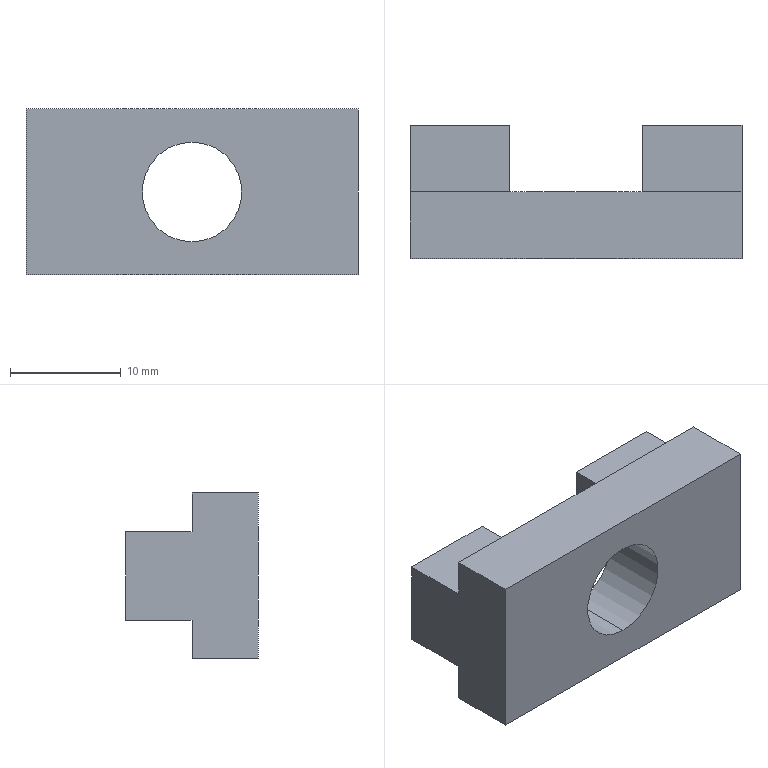Part | NX | features BREP 1 | 1 solid | 16 faces | box 30 x 12 x 15 mm | volume 3182 mm3 | plane 14 | cylinder 2 | commonest cylinder face diameters 9 x2
STEP:
#1=CARTESIAN_POINT('',(0.,6.,-4.5));
#2=VERTEX_POINT('',#1);
#3=CARTESIAN_POINT('',(0.,0.,-4.5));
#4=VERTEX_POINT('',#3);
#5=CARTESIAN_POINT('',(0.,0.,-4.5));
#6=DIRECTION('',(0.,1.,0.));
#7=VECTOR('',#6,1000.);
#8=LINE('',#5,#7);
#9=EDGE_CURVE('',#2,#4,#8,.F.);
#10=ORIENTED_EDGE('',*,*,#9,.T.);
#11=CARTESIAN_POINT('',(0.,0.,4.5));
#12=VERTEX_POINT('',#11);
#13=CARTESIAN_POINT('',(0.,0.,0.));
#14=DIRECTION('',(0.,1.,0.));
#15=DIRECTION('',(0.,0.,1.));
#16=AXIS2_PLACEMENT_3D('',#13,#14,#15);
#17=CIRCLE('',#16,4.5);
#18=EDGE_CURVE('',#12,#4,#17,.T.);
#19=ORIENTED_EDGE('',*,*,#18,.F.);
#20=CARTESIAN_POINT('',(0.,6.,4.5));
#21=VERTEX_POINT('',#20);
#22=CARTESIAN_POINT('',(0.,0.,4.5));
#23=DIRECTION('',(0.,1.,0.));
#24=VECTOR('',#23,1000.);
#25=LINE('',#22,#24);
#26=EDGE_CURVE('',#21,#12,#25,.F.);
#27=ORIENTED_EDGE('',*,*,#26,.F.);
#28=CARTESIAN_POINT('',(0.,6.,0.));
#29=DIRECTION('',(0.,1.,0.));
#30=DIRECTION('',(0.,0.,1.));
#31=AXIS2_PLACEMENT_3D('',#28,#29,#30);
#32=CIRCLE('',#31,4.5);
#33=EDGE_CURVE('',#21,#2,#32,.T.);
#34=ORIENTED_EDGE('',*,*,#33,.T.);
#35=EDGE_LOOP('',(#10,#19,#27,#34));
#36=FACE_BOUND('',#35,.T.);
#37=CARTESIAN_POINT('',(0.,0.,0.));
#38=DIRECTION('',(0.,1.,0.));
#39=DIRECTION('',(0.,0.,1.));
#40=AXIS2_PLACEMENT_3D('',#37,#38,#39);
#41=CYLINDRICAL_SURFACE('',#40,4.5);
#42=ADVANCED_FACE('',(#36),#41,.F.);
#43=CARTESIAN_POINT('',(-15.,6.,4.));
#44=VERTEX_POINT('',#43);
#45=CARTESIAN_POINT('',(-6.,6.,4.));
#46=VERTEX_POINT('',#45);
#47=CARTESIAN_POINT('',(-15.,6.,4.));
#48=DIRECTION('',(1.,0.,0.));
#49=VECTOR('',#48,1000.);
#50=LINE('',#47,#49);
#51=EDGE_CURVE('',#44,#46,#50,.T.);
#52=ORIENTED_EDGE('',*,*,#51,.T.);
#53=CARTESIAN_POINT('',(-6.,12.,4.));
#54=VERTEX_POINT('',#53);
#55=CARTESIAN_POINT('',(-6.,-3.657,4.));
#56=DIRECTION('',(0.,1.,0.));
#57=VECTOR('',#56,1000.);
#58=LINE('',#55,#57);
#59=EDGE_CURVE('',#46,#54,#58,.T.);
#60=ORIENTED_EDGE('',*,*,#59,.T.);
#61=CARTESIAN_POINT('',(-15.,12.,4.));
#62=VERTEX_POINT('',#61);
#63=CARTESIAN_POINT('',(-15.,12.,4.));
#64=DIRECTION('',(-1.,0.,0.));
#65=VECTOR('',#64,1000.);
#66=LINE('',#63,#65);
#67=EDGE_CURVE('',#54,#62,#66,.T.);
#68=ORIENTED_EDGE('',*,*,#67,.T.);
#69=CARTESIAN_POINT('',(-15.,-3.657,4.));
#70=DIRECTION('',(0.,1.,0.));
#71=VECTOR('',#70,1000.);
#72=LINE('',#69,#71);
#73=EDGE_CURVE('',#44,#62,#72,.T.);
#74=ORIENTED_EDGE('',*,*,#73,.F.);
#75=EDGE_LOOP('',(#52,#60,#68,#74));
#76=FACE_BOUND('',#75,.T.);
#77=CARTESIAN_POINT('',(-15.,-3.657,4.));
#78=DIRECTION('',(0.,0.,-1.));
#79=DIRECTION('',(-1.,0.,0.));
#80=AXIS2_PLACEMENT_3D('',#77,#78,#79);
#81=PLANE('',#80);
#82=ADVANCED_FACE('',(#76),#81,.F.);
#83=CARTESIAN_POINT('',(15.,6.,-4.));
#84=VERTEX_POINT('',#83);
#85=CARTESIAN_POINT('',(6.,6.,-4.));
#86=VERTEX_POINT('',#85);
#87=CARTESIAN_POINT('',(15.,6.,-4.));
#88=DIRECTION('',(-1.,0.,0.));
#89=VECTOR('',#88,1000.);
#90=LINE('',#87,#89);
#91=EDGE_CURVE('',#84,#86,#90,.T.);
#92=ORIENTED_EDGE('',*,*,#91,.T.);
#93=CARTESIAN_POINT('',(6.,12.,-4.));
#94=VERTEX_POINT('',#93);
#95=CARTESIAN_POINT('',(6.,-3.657,-4.));
#96=DIRECTION('',(0.,1.,0.));
#97=VECTOR('',#96,1000.);
#98=LINE('',#95,#97);
#99=EDGE_CURVE('',#86,#94,#98,.T.);
#100=ORIENTED_EDGE('',*,*,#99,.T.);
#101=CARTESIAN_POINT('',(15.,12.,-4.));
#102=VERTEX_POINT('',#101);
#103=CARTESIAN_POINT('',(15.,12.,-4.));
#104=DIRECTION('',(1.,0.,0.));
#105=VECTOR('',#104,1000.);
#106=LINE('',#103,#105);
#107=EDGE_CURVE('',#94,#102,#106,.T.);
#108=ORIENTED_EDGE('',*,*,#107,.T.);
#109=CARTESIAN_POINT('',(15.,-3.657,-4.));
#110=DIRECTION('',(0.,1.,0.));
#111=VECTOR('',#110,1000.);
#112=LINE('',#109,#111);
#113=EDGE_CURVE('',#84,#102,#112,.T.);
#114=ORIENTED_EDGE('',*,*,#113,.F.);
#115=EDGE_LOOP('',(#92,#100,#108,#114));
#116=FACE_BOUND('',#115,.T.);
#117=CARTESIAN_POINT('',(15.,-3.657,-4.));
#118=DIRECTION('',(0.,0.,1.));
#119=DIRECTION('',(1.,0.,0.));
#120=AXIS2_PLACEMENT_3D('',#117,#118,#119);
#121=PLANE('',#120);
#122=ADVANCED_FACE('',(#116),#121,.F.);
#123=CARTESIAN_POINT('',(6.,6.,4.));
#124=VERTEX_POINT('',#123);
#125=CARTESIAN_POINT('',(15.,6.,4.));
#126=VERTEX_POINT('',#125);
#127=CARTESIAN_POINT('',(15.,6.,4.));
#128=DIRECTION('',(1.,0.,0.));
#129=VECTOR('',#128,1000.);
#130=LINE('',#127,#129);
#131=EDGE_CURVE('',#124,#126,#130,.T.);
#132=ORIENTED_EDGE('',*,*,#131,.T.);
#133=CARTESIAN_POINT('',(15.,12.,4.));
#134=VERTEX_POINT('',#133);
#135=CARTESIAN_POINT('',(15.,-3.657,4.));
#136=DIRECTION('',(0.,1.,0.));
#137=VECTOR('',#136,1000.);
#138=LINE('',#135,#137);
#139=EDGE_CURVE('',#126,#134,#138,.T.);
#140=ORIENTED_EDGE('',*,*,#139,.T.);
#141=CARTESIAN_POINT('',(6.,12.,4.));
#142=VERTEX_POINT('',#141);
#143=CARTESIAN_POINT('',(15.,12.,4.));
#144=DIRECTION('',(-1.,0.,0.));
#145=VECTOR('',#144,1000.);
#146=LINE('',#143,#145);
#147=EDGE_CURVE('',#134,#142,#146,.T.);
#148=ORIENTED_EDGE('',*,*,#147,.T.);
#149=CARTESIAN_POINT('',(6.,-3.657,4.));
#150=DIRECTION('',(0.,1.,0.));
#151=VECTOR('',#150,1000.);
#152=LINE('',#149,#151);
#153=EDGE_CURVE('',#124,#142,#152,.T.);
#154=ORIENTED_EDGE('',*,*,#153,.F.);
#155=EDGE_LOOP('',(#132,#140,#148,#154));
#156=FACE_BOUND('',#155,.T.);
#157=CARTESIAN_POINT('',(15.,-3.657,4.));
#158=DIRECTION('',(0.,0.,-1.));
#159=DIRECTION('',(-1.,0.,0.));
#160=AXIS2_PLACEMENT_3D('',#157,#158,#159);
#161=PLANE('',#160);
#162=ADVANCED_FACE('',(#156),#161,.F.);
#163=CARTESIAN_POINT('',(-6.,6.,-4.));
#164=VERTEX_POINT('',#163);
#165=CARTESIAN_POINT('',(-15.,6.,-4.));
#166=VERTEX_POINT('',#165);
#167=CARTESIAN_POINT('',(-15.,6.,-4.));
#168=DIRECTION('',(-1.,0.,0.));
#169=VECTOR('',#168,1000.);
#170=LINE('',#167,#169);
#171=EDGE_CURVE('',#164,#166,#170,.T.);
#172=ORIENTED_EDGE('',*,*,#171,.T.);
#173=CARTESIAN_POINT('',(-15.,12.,-4.));
#174=VERTEX_POINT('',#173);
#175=CARTESIAN_POINT('',(-15.,-3.657,-4.));
#176=DIRECTION('',(0.,1.,0.));
#177=VECTOR('',#176,1000.);
#178=LINE('',#175,#177);
#179=EDGE_CURVE('',#166,#174,#178,.T.);
#180=ORIENTED_EDGE('',*,*,#179,.T.);
#181=CARTESIAN_POINT('',(-6.,12.,-4.));
#182=VERTEX_POINT('',#181);
#183=CARTESIAN_POINT('',(-15.,12.,-4.));
#184=DIRECTION('',(1.,0.,0.));
#185=VECTOR('',#184,1000.);
#186=LINE('',#183,#185);
#187=EDGE_CURVE('',#174,#182,#186,.T.);
#188=ORIENTED_EDGE('',*,*,#187,.T.);
#189=CARTESIAN_POINT('',(-6.,-3.657,-4.));
#190=DIRECTION('',(0.,1.,0.));
#191=VECTOR('',#190,1000.);
#192=LINE('',#189,#191);
#193=EDGE_CURVE('',#164,#182,#192,.T.);
#194=ORIENTED_EDGE('',*,*,#193,.F.);
#195=EDGE_LOOP('',(#172,#180,#188,#194));
#196=FACE_BOUND('',#195,.T.);
#197=CARTESIAN_POINT('',(-15.,-3.657,-4.));
#198=DIRECTION('',(0.,0.,1.));
#199=DIRECTION('',(1.,0.,0.));
#200=AXIS2_PLACEMENT_3D('',#197,#198,#199);
#201=PLANE('',#200);
#202=ADVANCED_FACE('',(#196),#201,.F.);
#203=CARTESIAN_POINT('',(15.,6.,-7.5));
#204=VERTEX_POINT('',#203);
#205=CARTESIAN_POINT('',(-15.,6.,-7.5));
#206=VERTEX_POINT('',#205);
#207=CARTESIAN_POINT('',(6.,6.,-7.5));
#208=DIRECTION('',(-1.,0.,0.));
#209=VECTOR('',#208,1000.);
#210=LINE('',#207,#209);
#211=EDGE_CURVE('',#204,#206,#210,.T.);
#212=ORIENTED_EDGE('',*,*,#211,.T.);
#213=CARTESIAN_POINT('',(-15.,6.,-7.5));
#214=DIRECTION('',(0.,0.,-1.));
#215=VECTOR('',#214,1000.);
#216=LINE('',#213,#215);
#217=EDGE_CURVE('',#166,#206,#216,.T.);
#218=ORIENTED_EDGE('',*,*,#217,.F.);
#219=ORIENTED_EDGE('',*,*,#171,.F.);
#220=CARTESIAN_POINT('',(-6.,6.,7.5));
#221=DIRECTION('',(0.,0.,1.));
#222=VECTOR('',#221,1000.);
#223=LINE('',#220,#222);
#224=EDGE_CURVE('',#164,#46,#223,.T.);
#225=ORIENTED_EDGE('',*,*,#224,.T.);
#226=ORIENTED_EDGE('',*,*,#51,.F.);
#227=CARTESIAN_POINT('',(-15.,6.,7.5));
#228=VERTEX_POINT('',#227);
#229=CARTESIAN_POINT('',(-15.,6.,7.5));
#230=DIRECTION('',(0.,0.,-1.));
#231=VECTOR('',#230,1000.);
#232=LINE('',#229,#231);
#233=EDGE_CURVE('',#228,#44,#232,.T.);
#234=ORIENTED_EDGE('',*,*,#233,.F.);
#235=CARTESIAN_POINT('',(15.,6.,7.5));
#236=VERTEX_POINT('',#235);
#237=CARTESIAN_POINT('',(6.,6.,7.5));
#238=DIRECTION('',(1.,0.,0.));
#239=VECTOR('',#238,1000.);
#240=LINE('',#237,#239);
#241=EDGE_CURVE('',#228,#236,#240,.T.);
#242=ORIENTED_EDGE('',*,*,#241,.T.);
#243=CARTESIAN_POINT('',(15.,6.,7.5));
#244=DIRECTION('',(0.,0.,1.));
#245=VECTOR('',#244,1000.);
#246=LINE('',#243,#245);
#247=EDGE_CURVE('',#126,#236,#246,.T.);
#248=ORIENTED_EDGE('',*,*,#247,.F.);
#249=ORIENTED_EDGE('',*,*,#131,.F.);
#250=CARTESIAN_POINT('',(6.,6.,7.5));
#251=DIRECTION('',(0.,0.,-1.));
#252=VECTOR('',#251,1000.);
#253=LINE('',#250,#252);
#254=EDGE_CURVE('',#124,#86,#253,.T.);
#255=ORIENTED_EDGE('',*,*,#254,.T.);
#256=ORIENTED_EDGE('',*,*,#91,.F.);
#257=CARTESIAN_POINT('',(15.,6.,-7.5));
#258=DIRECTION('',(0.,0.,1.));
#259=VECTOR('',#258,1000.);
#260=LINE('',#257,#259);
#261=EDGE_CURVE('',#204,#84,#260,.T.);
#262=ORIENTED_EDGE('',*,*,#261,.F.);
#263=EDGE_LOOP('',(#212,#218,#219,#225,#226,#234,#242,#248,#249,#255,#256,#262));
#264=FACE_BOUND('',#263,.T.);
#265=ORIENTED_EDGE('',*,*,#33,.F.);
#266=CARTESIAN_POINT('',(0.,6.,0.));
#267=DIRECTION('',(0.,1.,0.));
#268=DIRECTION('',(0.,0.,1.));
#269=AXIS2_PLACEMENT_3D('',#266,#267,#268);
#270=CIRCLE('',#269,4.5);
#271=EDGE_CURVE('',#2,#21,#270,.T.);
#272=ORIENTED_EDGE('',*,*,#271,.F.);
#273=EDGE_LOOP('',(#265,#272));
#274=FACE_BOUND('',#273,.T.);
#275=CARTESIAN_POINT('',(0.,6.,0.));
#276=DIRECTION('',(0.,1.,0.));
#277=DIRECTION('',(0.,0.,1.));
#278=AXIS2_PLACEMENT_3D('',#275,#276,#277);
#279=PLANE('',#278);
#280=ADVANCED_FACE('',(#264,#274),#279,.T.);
#281=CARTESIAN_POINT('',(6.,12.,7.5));
#282=DIRECTION('',(0.,0.,-1.));
#283=VECTOR('',#282,1000.);
#284=LINE('',#281,#283);
#285=EDGE_CURVE('',#142,#94,#284,.T.);
#286=ORIENTED_EDGE('',*,*,#285,.T.);
#287=ORIENTED_EDGE('',*,*,#99,.F.);
#288=ORIENTED_EDGE('',*,*,#254,.F.);
#289=ORIENTED_EDGE('',*,*,#153,.T.);
#290=EDGE_LOOP('',(#286,#287,#288,#289));
#291=FACE_BOUND('',#290,.T.);
#292=CARTESIAN_POINT('',(6.,6.,7.5));
#293=DIRECTION('',(1.,0.,0.));
#294=DIRECTION('',(0.,0.,-1.));
#295=AXIS2_PLACEMENT_3D('',#292,#293,#294);
#296=PLANE('',#295);
#297=ADVANCED_FACE('',(#291),#296,.F.);
#298=CARTESIAN_POINT('',(-6.,12.,7.5));
#299=DIRECTION('',(0.,0.,1.));
#300=VECTOR('',#299,1000.);
#301=LINE('',#298,#300);
#302=EDGE_CURVE('',#182,#54,#301,.T.);
#303=ORIENTED_EDGE('',*,*,#302,.T.);
#304=ORIENTED_EDGE('',*,*,#59,.F.);
#305=ORIENTED_EDGE('',*,*,#224,.F.);
#306=ORIENTED_EDGE('',*,*,#193,.T.);
#307=EDGE_LOOP('',(#303,#304,#305,#306));
#308=FACE_BOUND('',#307,.T.);
#309=CARTESIAN_POINT('',(-6.,6.,7.5));
#310=DIRECTION('',(-1.,0.,0.));
#311=DIRECTION('',(0.,0.,1.));
#312=AXIS2_PLACEMENT_3D('',#309,#310,#311);
#313=PLANE('',#312);
#314=ADVANCED_FACE('',(#308),#313,.F.);
#315=CARTESIAN_POINT('',(-15.,0.,-7.5));
#316=VERTEX_POINT('',#315);
#317=CARTESIAN_POINT('',(-15.,0.,7.5));
#318=VERTEX_POINT('',#317);
#319=CARTESIAN_POINT('',(-15.,0.,7.5));
#320=DIRECTION('',(0.,0.,1.));
#321=VECTOR('',#320,1000.);
#322=LINE('',#319,#321);
#323=EDGE_CURVE('',#316,#318,#322,.T.);
#324=ORIENTED_EDGE('',*,*,#323,.F.);
#325=CARTESIAN_POINT('',(15.,0.,-7.5));
#326=VERTEX_POINT('',#325);
#327=CARTESIAN_POINT('',(15.,0.,-7.5));
#328=DIRECTION('',(-1.,0.,0.));
#329=VECTOR('',#328,1000.);
#330=LINE('',#327,#329);
#331=EDGE_CURVE('',#326,#316,#330,.T.);
#332=ORIENTED_EDGE('',*,*,#331,.F.);
#333=CARTESIAN_POINT('',(15.,0.,7.5));
#334=VERTEX_POINT('',#333);
#335=CARTESIAN_POINT('',(15.,0.,7.5));
#336=DIRECTION('',(0.,0.,-1.));
#337=VECTOR('',#336,1000.);
#338=LINE('',#335,#337);
#339=EDGE_CURVE('',#334,#326,#338,.T.);
#340=ORIENTED_EDGE('',*,*,#339,.F.);
#341=CARTESIAN_POINT('',(15.,0.,7.5));
#342=DIRECTION('',(1.,0.,0.));
#343=VECTOR('',#342,1000.);
#344=LINE('',#341,#343);
#345=EDGE_CURVE('',#318,#334,#344,.T.);
#346=ORIENTED_EDGE('',*,*,#345,.F.);
#347=EDGE_LOOP('',(#324,#332,#340,#346));
#348=FACE_BOUND('',#347,.T.);
#349=ORIENTED_EDGE('',*,*,#18,.T.);
#350=CARTESIAN_POINT('',(0.,0.,0.));
#351=DIRECTION('',(0.,1.,0.));
#352=DIRECTION('',(0.,0.,1.));
#353=AXIS2_PLACEMENT_3D('',#350,#351,#352);
#354=CIRCLE('',#353,4.5);
#355=EDGE_CURVE('',#4,#12,#354,.T.);
#356=ORIENTED_EDGE('',*,*,#355,.T.);
#357=EDGE_LOOP('',(#349,#356));
#358=FACE_BOUND('',#357,.T.);
#359=CARTESIAN_POINT('',(0.,0.,0.));
#360=DIRECTION('',(0.,1.,0.));
#361=DIRECTION('',(0.,0.,1.));
#362=AXIS2_PLACEMENT_3D('',#359,#360,#361);
#363=PLANE('',#362);
#364=ADVANCED_FACE('',(#348,#358),#363,.F.);
#365=ORIENTED_EDGE('',*,*,#107,.F.);
#366=ORIENTED_EDGE('',*,*,#285,.F.);
#367=ORIENTED_EDGE('',*,*,#147,.F.);
#368=CARTESIAN_POINT('',(15.,12.,7.5));
#369=DIRECTION('',(0.,0.,-1.));
#370=VECTOR('',#369,1000.);
#371=LINE('',#368,#370);
#372=EDGE_CURVE('',#134,#102,#371,.T.);
#373=ORIENTED_EDGE('',*,*,#372,.T.);
#374=EDGE_LOOP('',(#365,#366,#367,#373));
#375=FACE_BOUND('',#374,.T.);
#376=CARTESIAN_POINT('',(0.,12.,0.));
#377=DIRECTION('',(0.,1.,0.));
#378=DIRECTION('',(0.,0.,1.));
#379=AXIS2_PLACEMENT_3D('',#376,#377,#378);
#380=PLANE('',#379);
#381=ADVANCED_FACE('',(#375),#380,.T.);
#382=ORIENTED_EDGE('',*,*,#261,.T.);
#383=ORIENTED_EDGE('',*,*,#113,.T.);
#384=ORIENTED_EDGE('',*,*,#372,.F.);
#385=ORIENTED_EDGE('',*,*,#139,.F.);
#386=ORIENTED_EDGE('',*,*,#247,.T.);
#387=CARTESIAN_POINT('',(15.,12.,7.5));
#388=DIRECTION('',(0.,-1.,0.));
#389=VECTOR('',#388,1000.);
#390=LINE('',#387,#389);
#391=EDGE_CURVE('',#236,#334,#390,.T.);
#392=ORIENTED_EDGE('',*,*,#391,.T.);
#393=ORIENTED_EDGE('',*,*,#339,.T.);
#394=CARTESIAN_POINT('',(15.,12.,-7.5));
#395=DIRECTION('',(0.,-1.,0.));
#396=VECTOR('',#395,1000.);
#397=LINE('',#394,#396);
#398=EDGE_CURVE('',#204,#326,#397,.T.);
#399=ORIENTED_EDGE('',*,*,#398,.F.);
#400=EDGE_LOOP('',(#382,#383,#384,#385,#386,#392,#393,#399));
#401=FACE_BOUND('',#400,.T.);
#402=CARTESIAN_POINT('',(15.,12.,7.5));
#403=DIRECTION('',(-1.,0.,0.));
#404=DIRECTION('',(0.,0.,1.));
#405=AXIS2_PLACEMENT_3D('',#402,#403,#404);
#406=PLANE('',#405);
#407=ADVANCED_FACE('',(#401),#406,.F.);
#408=ORIENTED_EDGE('',*,*,#233,.T.);
#409=ORIENTED_EDGE('',*,*,#73,.T.);
#410=CARTESIAN_POINT('',(-15.,12.,7.5));
#411=DIRECTION('',(0.,0.,1.));
#412=VECTOR('',#411,1000.);
#413=LINE('',#410,#412);
#414=EDGE_CURVE('',#174,#62,#413,.T.);
#415=ORIENTED_EDGE('',*,*,#414,.F.);
#416=ORIENTED_EDGE('',*,*,#179,.F.);
#417=ORIENTED_EDGE('',*,*,#217,.T.);
#418=CARTESIAN_POINT('',(-15.,12.,-7.5));
#419=DIRECTION('',(0.,-1.,0.));
#420=VECTOR('',#419,1000.);
#421=LINE('',#418,#420);
#422=EDGE_CURVE('',#206,#316,#421,.T.);
#423=ORIENTED_EDGE('',*,*,#422,.T.);
#424=ORIENTED_EDGE('',*,*,#323,.T.);
#425=CARTESIAN_POINT('',(-15.,12.,7.5));
#426=DIRECTION('',(0.,-1.,0.));
#427=VECTOR('',#426,1000.);
#428=LINE('',#425,#427);
#429=EDGE_CURVE('',#228,#318,#428,.T.);
#430=ORIENTED_EDGE('',*,*,#429,.F.);
#431=EDGE_LOOP('',(#408,#409,#415,#416,#417,#423,#424,#430));
#432=FACE_BOUND('',#431,.T.);
#433=CARTESIAN_POINT('',(-15.,12.,7.5));
#434=DIRECTION('',(1.,0.,0.));
#435=DIRECTION('',(0.,0.,-1.));
#436=AXIS2_PLACEMENT_3D('',#433,#434,#435);
#437=PLANE('',#436);
#438=ADVANCED_FACE('',(#432),#437,.F.);
#439=ORIENTED_EDGE('',*,*,#67,.F.);
#440=ORIENTED_EDGE('',*,*,#302,.F.);
#441=ORIENTED_EDGE('',*,*,#187,.F.);
#442=ORIENTED_EDGE('',*,*,#414,.T.);
#443=EDGE_LOOP('',(#439,#440,#441,#442));
#444=FACE_BOUND('',#443,.T.);
#445=CARTESIAN_POINT('',(0.,12.,0.));
#446=DIRECTION('',(0.,1.,0.));
#447=DIRECTION('',(0.,0.,1.));
#448=AXIS2_PLACEMENT_3D('',#445,#446,#447);
#449=PLANE('',#448);
#450=ADVANCED_FACE('',(#444),#449,.T.);
#451=ORIENTED_EDGE('',*,*,#211,.F.);
#452=ORIENTED_EDGE('',*,*,#398,.T.);
#453=ORIENTED_EDGE('',*,*,#331,.T.);
#454=ORIENTED_EDGE('',*,*,#422,.F.);
#455=EDGE_LOOP('',(#451,#452,#453,#454));
#456=FACE_BOUND('',#455,.T.);
#457=CARTESIAN_POINT('',(15.,12.,-7.5));
#458=DIRECTION('',(0.,0.,1.));
#459=DIRECTION('',(1.,0.,0.));
#460=AXIS2_PLACEMENT_3D('',#457,#458,#459);
#461=PLANE('',#460);
#462=ADVANCED_FACE('',(#456),#461,.F.);
#463=ORIENTED_EDGE('',*,*,#241,.F.);
#464=ORIENTED_EDGE('',*,*,#429,.T.);
#465=ORIENTED_EDGE('',*,*,#345,.T.);
#466=ORIENTED_EDGE('',*,*,#391,.F.);
#467=EDGE_LOOP('',(#463,#464,#465,#466));
#468=FACE_BOUND('',#467,.T.);
#469=CARTESIAN_POINT('',(15.,12.,7.5));
#470=DIRECTION('',(0.,0.,-1.));
#471=DIRECTION('',(-1.,0.,0.));
#472=AXIS2_PLACEMENT_3D('',#469,#470,#471);
#473=PLANE('',#472);
#474=ADVANCED_FACE('',(#468),#473,.F.);
#475=ORIENTED_EDGE('',*,*,#355,.F.);
#476=ORIENTED_EDGE('',*,*,#9,.F.);
#477=ORIENTED_EDGE('',*,*,#271,.T.);
#478=ORIENTED_EDGE('',*,*,#26,.T.);
#479=EDGE_LOOP('',(#475,#476,#477,#478));
#480=FACE_BOUND('',#479,.T.);
#481=CARTESIAN_POINT('',(0.,0.,0.));
#482=DIRECTION('',(0.,1.,0.));
#483=DIRECTION('',(0.,0.,1.));
#484=AXIS2_PLACEMENT_3D('',#481,#482,#483);
#485=CYLINDRICAL_SURFACE('',#484,4.5);
#486=ADVANCED_FACE('',(#480),#485,.F.);
#487=CLOSED_SHELL('',(#42,#82,#122,#162,#202,#280,#297,#314,#364,#381,#407,#438,#450,#462,#474,#486));
#488=MANIFOLD_SOLID_BREP('',#487);
#489=(LENGTH_UNIT()NAMED_UNIT(*)SI_UNIT(.MILLI.,.METRE.));
#490=UNCERTAINTY_MEASURE_WITH_UNIT(LENGTH_MEASURE(0.00001),#489,'','');
#491=(NAMED_UNIT(*)PLANE_ANGLE_UNIT()SI_UNIT($,.RADIAN.));
#492=(NAMED_UNIT(*)SI_UNIT($,.STERADIAN.)SOLID_ANGLE_UNIT());
#493=(GEOMETRIC_REPRESENTATION_CONTEXT(3)GLOBAL_UNCERTAINTY_ASSIGNED_CONTEXT((#490))GLOBAL_UNIT_ASSIGNED_CONTEXT((#489,#491,#492))REPRESENTATION_CONTEXT('',''));
#494=ADVANCED_BREP_SHAPE_REPRESENTATION('',(#488),#493);